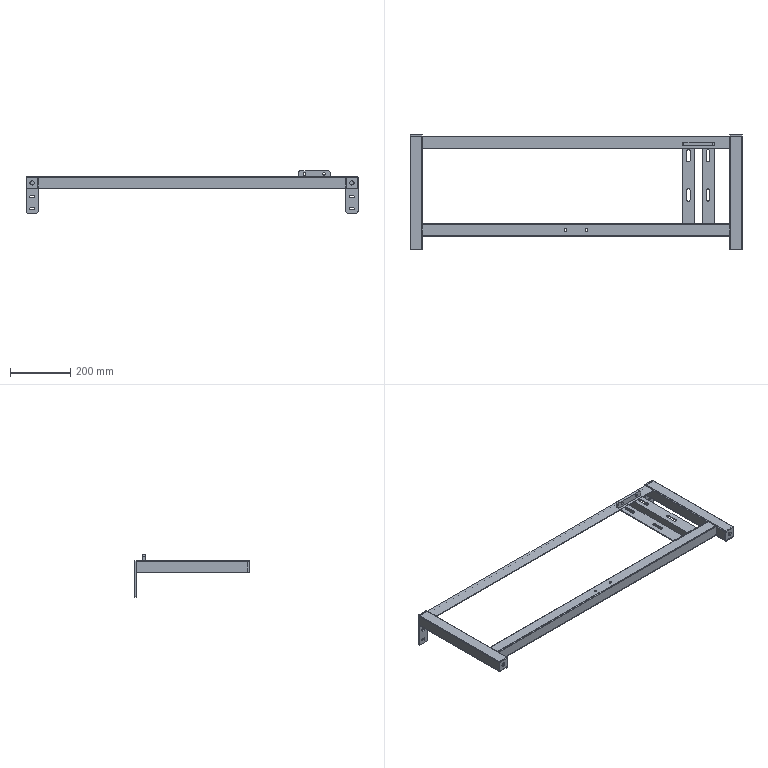Part | SolidWorks | features BaseBody 11 | 11 solids | 195 faces | box 1100 x 380 x 140 mm | volume 876113 mm3 | plane 106 | cylinder 89 | commonest cylinder face diameters 9 x22 6 x20 10 x13 3 x12 11 x8 2.667 x4